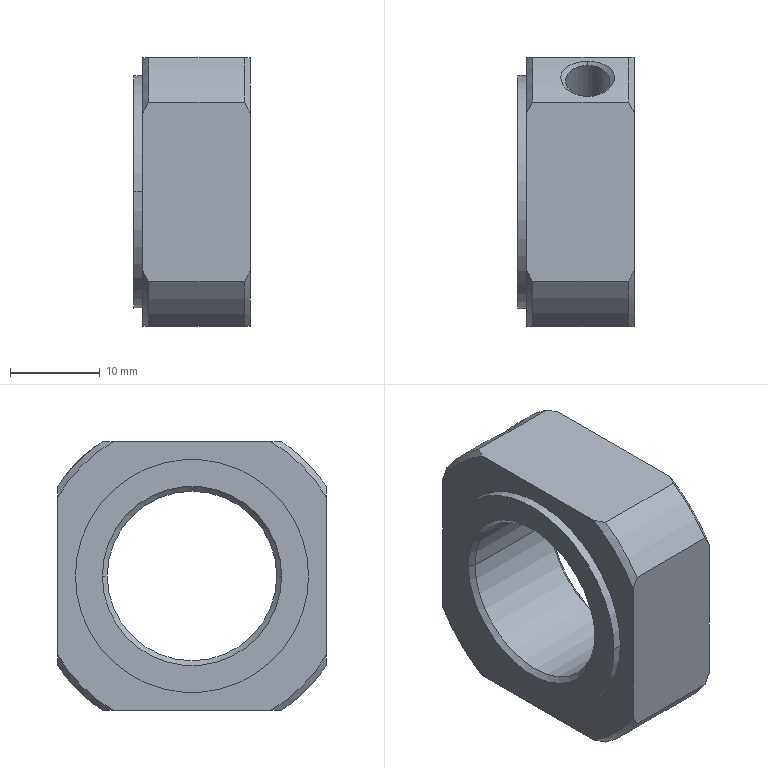Part | NX | 1 solid | 31 faces | box 13 x 30 x 30 mm | volume 6962 mm3 | cone 14 | cylinder 10 | plane 7 | commonest cylinder face diameters 36.062 x4 4.917 x2 18.917 x2 26 x2